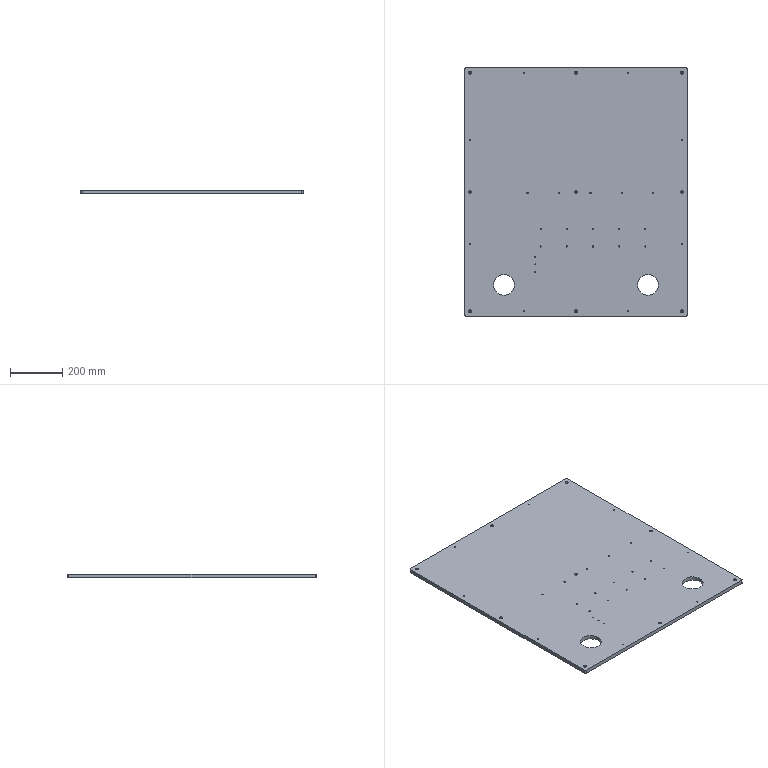Part | SolidWorks | features HoleWzd 5, Cut 1, Extrusion 1, Fillet 1, LPattern 1 | 1 solid | 111 faces | box 850 x 950 x 15 mm | volume 11946510 mm3 | cylinder 96 | plane 15 | commonest cylinder face diameters 4.2 x26 5 x26 6.6 x18 11 x18 10 x4 80 x4